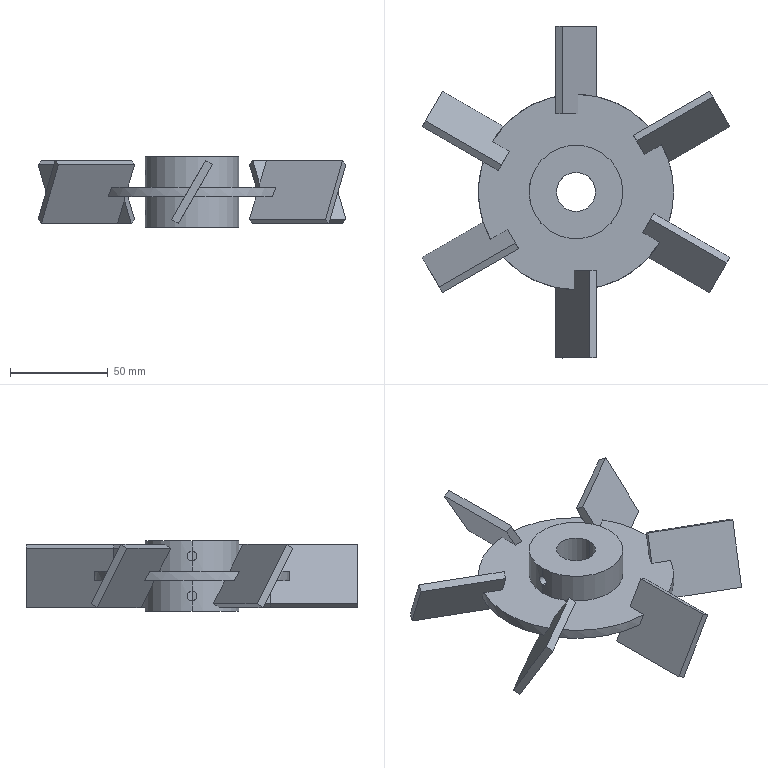Part | SolidWorks | features ICE 4, 3DProfileFeature 2, BaseBody 1, CirPattern 1, HoleWzd 1, Scale 1 | 1 solid | 66 faces | box 157.706 x 170 x 36 mm | volume 118469 mm3 | plane 47 | cylinder 19 | commonest cylinder face diameters 100 x7 5 x4 48 x4 20 x2 24 x2